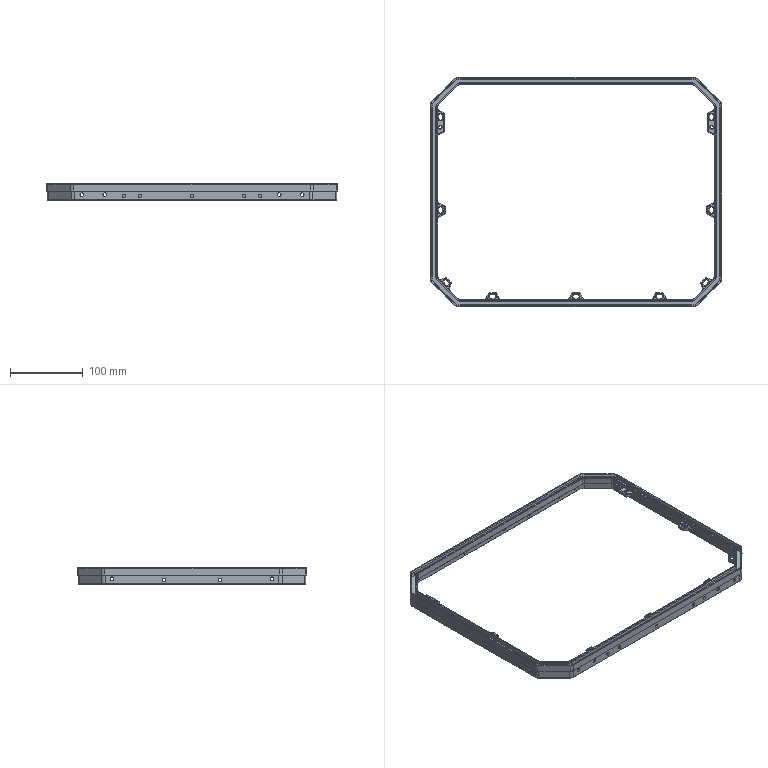Part | SolidWorks | features BaseBody 1 | 1 solid | 621 faces | box 400 x 315 x 22.5 mm | volume 130100 mm3 | cylinder 289 | plane 146 | torus 106 | cone 44 | spline 36 | commonest cylinder face diameters 2 x105 4.9 x50 8 x26 4 x24 5 x24 1 x16